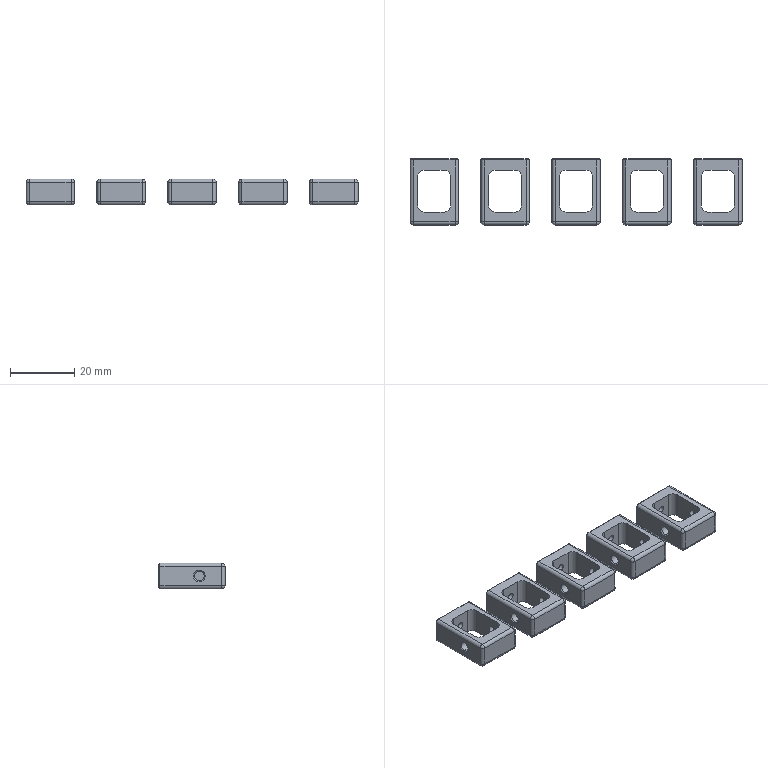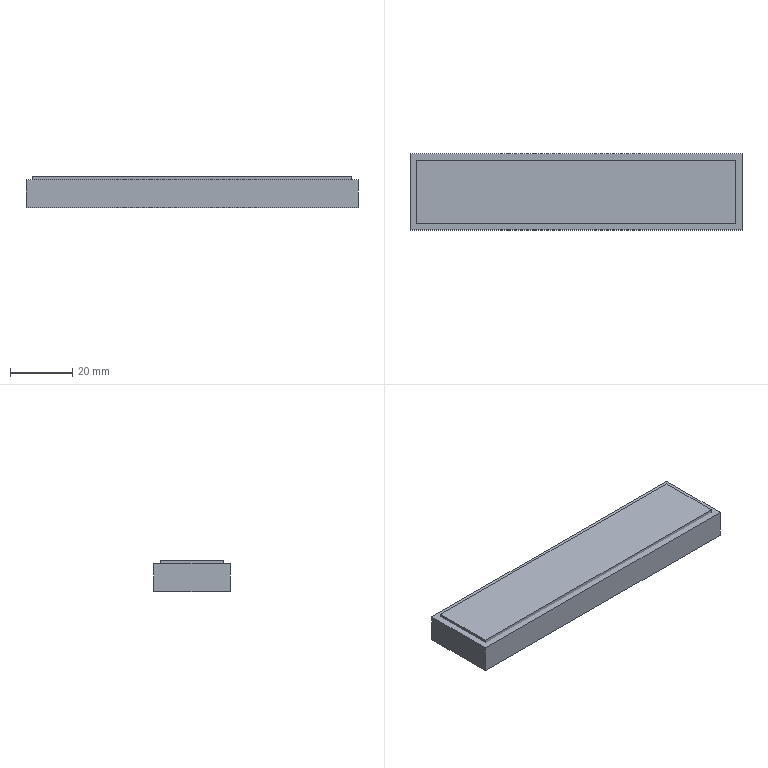CAM job | NX | 3-axis milling | part box 103 x 20.5 x 8 mm | stock box 107 x 24.5 x 10 mm
Tools:
number,name,description,diameter,corner_radius,flute_length,length,flutes
19,D80,Milling Tool-5 Parameters,80.0,0.0,50.0,75.0,2
12,D6,Milling Tool-5 Parameters,6.0,0.0,50.0,75.0,2
11,D4,Milling Tool-5 Parameters,4.0,0.0,50.0,75.0,2
1,D6A45,Milling Tool-5 Parameters,6.0,0.0,50.0,75.0,2
16,D4R0.5,Milling Tool-5 Parameters,4.0,0.5,50.0,75.0,2
Operations:
program,operation,operation_type,tool,method,geometry_group,spindle_rpm,surface_speed,feed_per_tooth,feed_cut,feed_plunge,cut_length_mm,path_length_mm,cut_time_min,machine_time_min
1,FLOOR_WALL,VolumeBased25DMillingOperation,D80,METHOD,A,6500.0,1633.0,0.1154,1500.0,100.0,199.0,253.0,0.1327,0.1381
1,ZLEVEL_PROFILE,ZLevelMilling,D6,METHOD,A,9500.0,298.0,0.1579,3000.0,1000.0,8725.737,10144.053,3.172,3.314
1,ZLEVEL_PROFILE_COPY,ZLevelMilling,D6,METHOD,A,9500.0,298.0,0.0789,1500.0,1000.0,582.971,2073.102,0.3933,0.5423
1,ZLEVEL_PROFILE_COPY_1,ZLevelMilling,D4,METHOD,A,9950.0,125.0,0.0804,1600.0,1000.0,2249.082,4584.508,1.653,1.887
1,PLANAR_MILL_COPY,PlanarMilling,D6A45,METHOD,A,9500.0,179.0,0.0658,1250.0,100.0,220.112,609.551,0.1761,0.215
1,ZLEVEL_PROFILE_1,ZLevelMilling,D4R0.5,METHOD,A,9500.0,119.0,0.1579,3000.0,100.0,7994.771,8235.442,2.665,2.689
2,FLOOR_WALL_COPY,VolumeBased25DMillingOperation,D80,METHOD,B,6500.0,1633.0,0.1154,1500.0,100.0,390.0,685,0.26,0.2895
2,PLANAR_MILL_COPY_COPY,PlanarMilling,D6A45,METHOD,B,9500.0,179.0,0.0658,1250.0,100.0,220.112,609.551,0.1761,0.215
2,ZLEVEL_PROFILE_1_COPY,ZLevelMilling,D4R0.5,METHOD,B,9500.0,119.0,0.1579,3000.0,100.0,7994.767,8235.438,2.665,2.689